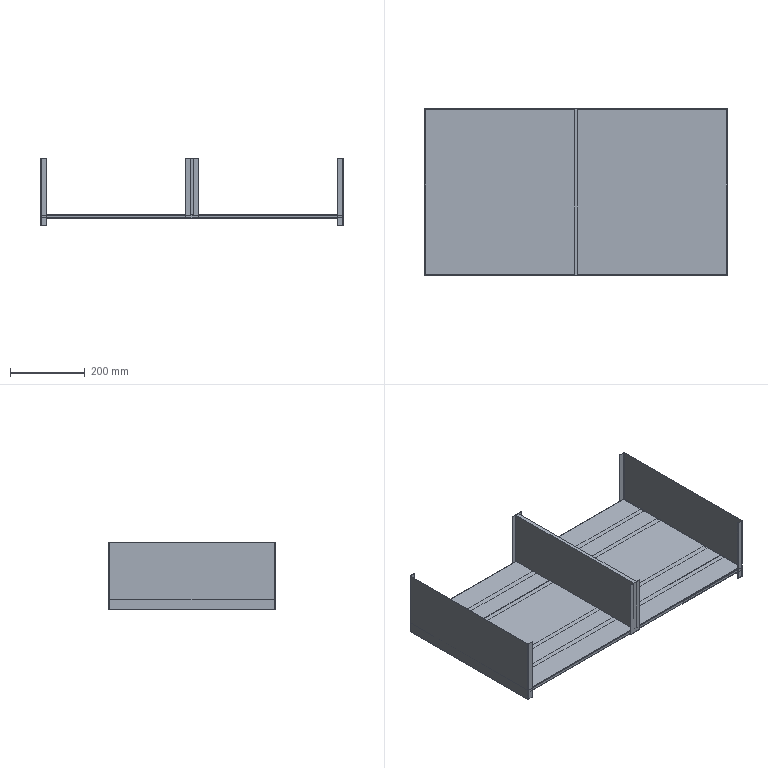Part | SolidWorks | features BaseBody 8 | 8 solids | 180 faces | box 809.4 x 448 x 181.2 mm | volume 1546539 mm3 | plane 148 | cylinder 32 | commonest cylinder face diameters 2 x16 4.4 x16